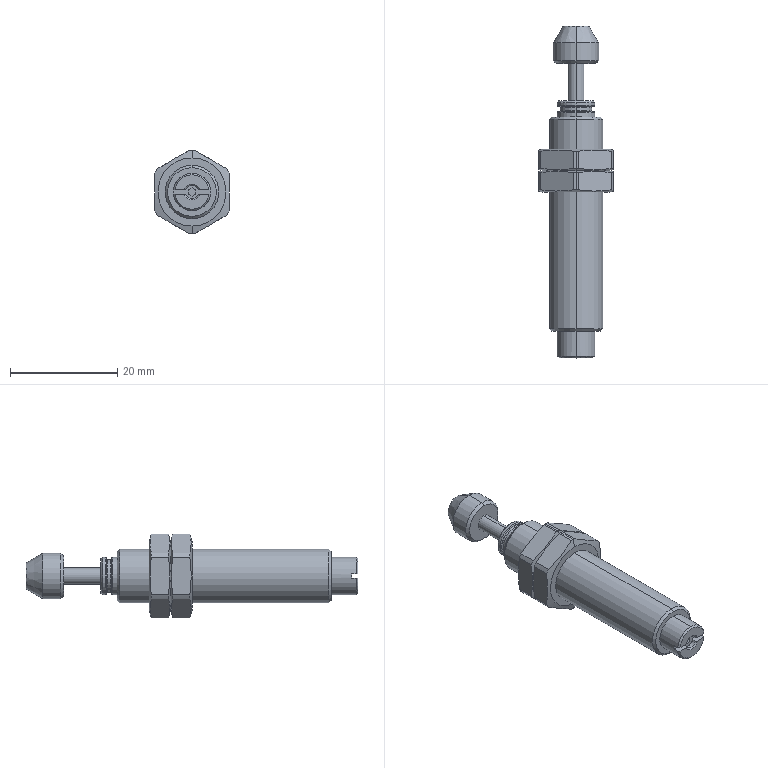Part | STEP file | Hydraulic shock absorber ACA1007-2 | 3 solids | 112 faces | box 14 x 62 x 15.686 mm | volume 4586 mm3 | plane 37 | cylinder 34 | cone 33 | torus 8 | commonest cylinder face diameters 15.686 x14 7 x6 9.188 x4 2.459 x2 3 x2 6 x2